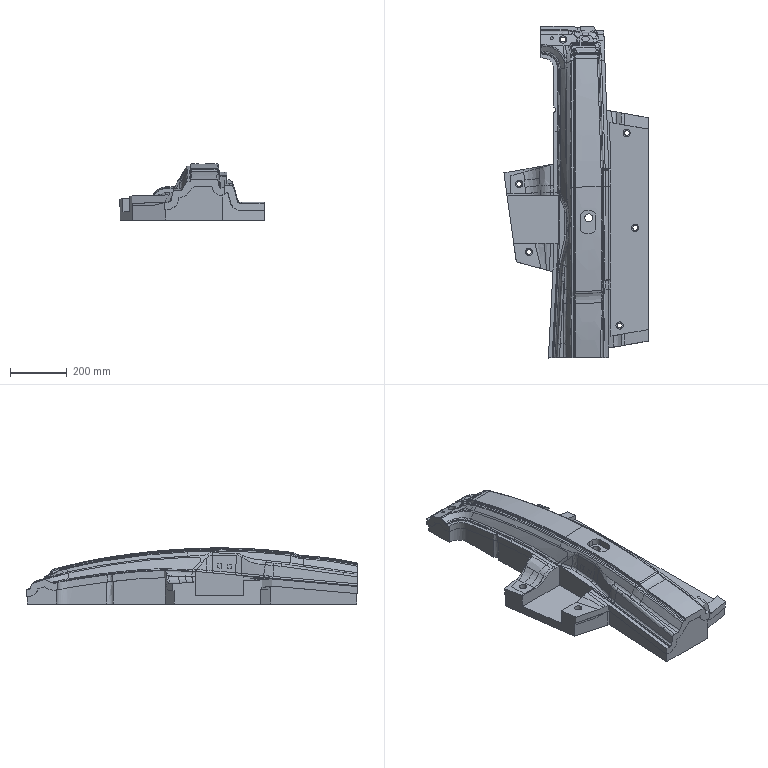Part | NX | features solid 2 | 1 solid | 424 faces | box 509.678 x 1173 x 198.441 mm | volume 41678562 mm3 | spline 357 | plane 43 | cylinder 24 | commonest cylinder face diameters 17 x6 26 x6 32 x6 40 x4 10 x1 28 x1